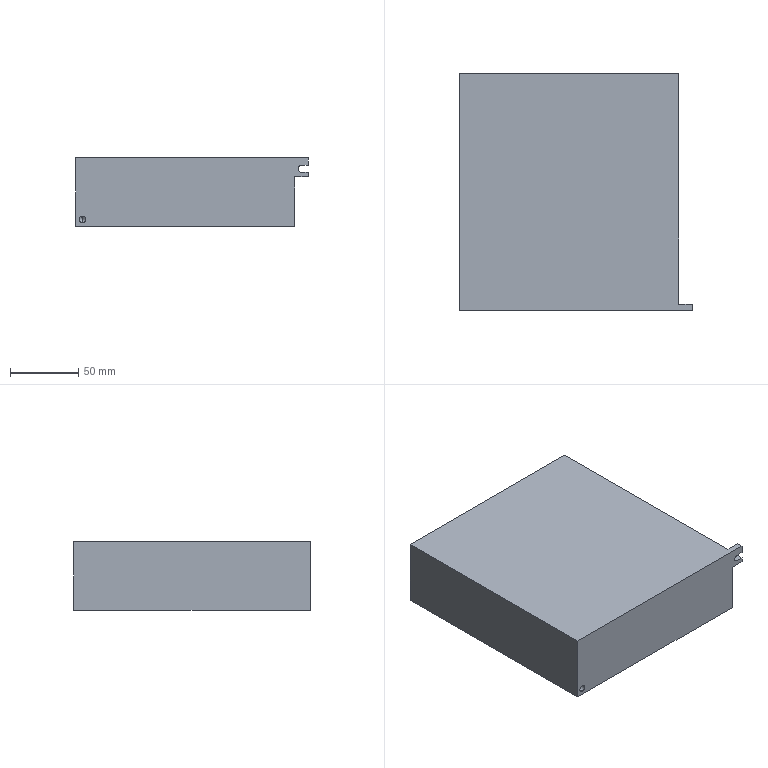Part | STEP file | Jiemeikang 750W driver | 1 solid | 17 faces | box 170 x 173 x 50 mm | volume 1384193 mm3 | plane 12 | cylinder 3 | cone 2 | commonest cylinder face diameters 4.8 x2 5 x1
STEP:
#1=CARTESIAN_POINT('',(0.,0.,0.));
#2=DIRECTION('',(0.,0.,1.));
#3=DIRECTION('',(1.,0.,0.));
#4=AXIS2_PLACEMENT_3D('',#1,#2,#3);
#5=CARTESIAN_POINT('',(-75.,15.,-22.4));
#6=VERTEX_POINT('',#5);
#7=CARTESIAN_POINT('',(-75.,0.,-22.4));
#8=VERTEX_POINT('',#7);
#9=CARTESIAN_POINT('',(-75.,0.,-22.4));
#10=DIRECTION('',(0.,-1.,0.));
#11=VECTOR('',#10,1.);
#12=LINE('',#9,#11);
#13=CARTESIAN_POINT('',(-75.,0.,-20.));
#14=DIRECTION('',(0.,-1.,0.));
#15=DIRECTION('',(0.,0.,-1.));
#16=AXIS2_PLACEMENT_3D('',#13,#14,#15);
#17=CYLINDRICAL_SURFACE('',#16,2.4);
#18=CARTESIAN_POINT('',(6.283,0.));
#19=DIRECTION('',(0.,1.));
#20=VECTOR('',#19,1.);
#21=LINE('',#18,#20);
#22=(GEOMETRIC_REPRESENTATION_CONTEXT(2)PARAMETRIC_REPRESENTATION_CONTEXT()REPRESENTATION_CONTEXT('',''));
#23=DEFINITIONAL_REPRESENTATION('',(#21),#22);
#24=PCURVE('',#17,#23);
#25=CARTESIAN_POINT('',(-75.,0.,-20.));
#26=DIRECTION('',(0.,-1.,0.));
#27=DIRECTION('',(0.,0.,-1.));
#28=AXIS2_PLACEMENT_3D('',#25,#26,#27);
#29=CYLINDRICAL_SURFACE('',#28,2.4);
#30=CARTESIAN_POINT('',(0.,0.));
#31=DIRECTION('',(0.,1.));
#32=VECTOR('',#31,1.);
#33=LINE('',#30,#32);
#34=(GEOMETRIC_REPRESENTATION_CONTEXT(2)PARAMETRIC_REPRESENTATION_CONTEXT()REPRESENTATION_CONTEXT('',''));
#35=DEFINITIONAL_REPRESENTATION('',(#33),#34);
#36=PCURVE('',#29,#35);
#37=SURFACE_CURVE('',#12,(#24,#36),.PCURVE_S1.);
#38=EDGE_CURVE('',#6,#8,#37,.T.);
#39=ORIENTED_EDGE('',*,*,#38,.T.);
#40=CARTESIAN_POINT('',(-75.,0.,-17.6));
#41=VERTEX_POINT('',#40);
#42=CARTESIAN_POINT('',(-75.,0.,-20.));
#43=DIRECTION('',(0.,-1.,0.));
#44=DIRECTION('',(0.,0.,-1.));
#45=AXIS2_PLACEMENT_3D('',#42,#43,#44);
#46=CIRCLE('',#45,2.4);
#47=CARTESIAN_POINT('',(0.,0.));
#48=DIRECTION('',(1.,0.));
#49=VECTOR('',#48,1.);
#50=LINE('',#47,#49);
#51=(GEOMETRIC_REPRESENTATION_CONTEXT(2)PARAMETRIC_REPRESENTATION_CONTEXT()REPRESENTATION_CONTEXT('',''));
#52=DEFINITIONAL_REPRESENTATION('',(#50),#51);
#53=PCURVE('',#17,#52);
#54=CARTESIAN_POINT('',(0.,0.,0.));
#55=DIRECTION('',(0.,-1.,0.));
#56=DIRECTION('',(0.,0.,-1.));
#57=AXIS2_PLACEMENT_3D('',#54,#55,#56);
#58=PLANE('',#57);
#59=CARTESIAN_POINT('',(20.,-75.));
#60=DIRECTION('',(1.,0.));
#61=AXIS2_PLACEMENT_2D('',#59,#60);
#62=CIRCLE('',#61,2.4);
#63=(GEOMETRIC_REPRESENTATION_CONTEXT(2)PARAMETRIC_REPRESENTATION_CONTEXT()REPRESENTATION_CONTEXT('',''));
#64=DEFINITIONAL_REPRESENTATION('',(#62),#63);
#65=PCURVE('',#58,#64);
#66=SURFACE_CURVE('',#46,(#53,#65),.PCURVE_S1.);
#67=EDGE_CURVE('',#41,#8,#66,.T.);
#68=ORIENTED_EDGE('',*,*,#67,.F.);
#69=CARTESIAN_POINT('',(-75.,15.,-17.6));
#70=VERTEX_POINT('',#69);
#71=CARTESIAN_POINT('',(-75.,0.,-17.6));
#72=DIRECTION('',(0.,-1.,0.));
#73=VECTOR('',#72,1.);
#74=LINE('',#71,#73);
#75=CARTESIAN_POINT('',(3.142,0.));
#76=DIRECTION('',(0.,1.));
#77=VECTOR('',#76,1.);
#78=LINE('',#75,#77);
#79=(GEOMETRIC_REPRESENTATION_CONTEXT(2)PARAMETRIC_REPRESENTATION_CONTEXT()REPRESENTATION_CONTEXT('',''));
#80=DEFINITIONAL_REPRESENTATION('',(#78),#79);
#81=PCURVE('',#17,#80);
#82=CARTESIAN_POINT('',(3.142,0.));
#83=DIRECTION('',(0.,1.));
#84=VECTOR('',#83,1.);
#85=LINE('',#82,#84);
#86=(GEOMETRIC_REPRESENTATION_CONTEXT(2)PARAMETRIC_REPRESENTATION_CONTEXT()REPRESENTATION_CONTEXT('',''));
#87=DEFINITIONAL_REPRESENTATION('',(#85),#86);
#88=PCURVE('',#29,#87);
#89=SURFACE_CURVE('',#74,(#81,#88),.PCURVE_S1.);
#90=EDGE_CURVE('',#70,#41,#89,.T.);
#91=ORIENTED_EDGE('',*,*,#90,.F.);
#92=CARTESIAN_POINT('',(-75.,15.,-20.));
#93=DIRECTION('',(0.,-1.,0.));
#94=DIRECTION('',(0.,0.,-1.));
#95=AXIS2_PLACEMENT_3D('',#92,#93,#94);
#96=CIRCLE('',#95,2.4);
#97=CARTESIAN_POINT('',(0.,-15.));
#98=DIRECTION('',(1.,0.));
#99=VECTOR('',#98,1.);
#100=LINE('',#97,#99);
#101=(GEOMETRIC_REPRESENTATION_CONTEXT(2)PARAMETRIC_REPRESENTATION_CONTEXT()REPRESENTATION_CONTEXT('',''));
#102=DEFINITIONAL_REPRESENTATION('',(#100),#101);
#103=PCURVE('',#17,#102);
#104=CARTESIAN_POINT('',(-75.,15.,-20.));
#105=DIRECTION('',(0.,-1.,0.));
#106=DIRECTION('',(0.,0.,-1.));
#107=AXIS2_PLACEMENT_3D('',#104,#105,#106);
#108=CONICAL_SURFACE('',#107,2.4,1.03);
#109=CARTESIAN_POINT('',(0.,0.));
#110=DIRECTION('',(1.,0.));
#111=VECTOR('',#110,1.);
#112=LINE('',#109,#111);
#113=(GEOMETRIC_REPRESENTATION_CONTEXT(2)PARAMETRIC_REPRESENTATION_CONTEXT()REPRESENTATION_CONTEXT('',''));
#114=DEFINITIONAL_REPRESENTATION('',(#112),#113);
#115=PCURVE('',#108,#114);
#116=SURFACE_CURVE('',#96,(#103,#115),.PCURVE_S1.);
#117=EDGE_CURVE('',#70,#6,#116,.T.);
#118=ORIENTED_EDGE('',*,*,#117,.T.);
#119=EDGE_LOOP('',(#39,#68,#91,#118));
#120=FACE_BOUND('',#119,.F.);
#121=ADVANCED_FACE('',(#120),#17,.F.);
#122=ORIENTED_EDGE('',*,*,#117,.F.);
#123=CARTESIAN_POINT('',(-75.,16.442,-20.));
#124=VERTEX_POINT('',#123);
#125=CARTESIAN_POINT('',(-75.,15.,-17.6));
#126=DIRECTION('',(0.,-0.515,0.8572));
#127=VECTOR('',#126,1.);
#128=LINE('',#125,#127);
#129=CARTESIAN_POINT('',(3.142,-1.442));
#130=CARTESIAN_POINT('',(3.142,-1.42));
#131=CARTESIAN_POINT('',(3.142,-1.377));
#132=CARTESIAN_POINT('',(3.142,-1.311));
#133=CARTESIAN_POINT('',(3.142,-1.245));
#134=CARTESIAN_POINT('',(3.142,-1.18));
#135=CARTESIAN_POINT('',(3.142,-1.114));
#136=CARTESIAN_POINT('',(3.142,-1.049));
#137=CARTESIAN_POINT('',(3.142,-0.9832));
#138=CARTESIAN_POINT('',(3.142,-0.9177));
#139=CARTESIAN_POINT('',(3.142,-0.8521));
#140=CARTESIAN_POINT('',(3.142,-0.7866));
#141=CARTESIAN_POINT('',(3.142,-0.721));
#142=CARTESIAN_POINT('',(3.142,-0.6555));
#143=CARTESIAN_POINT('',(3.142,-0.5899));
#144=CARTESIAN_POINT('',(3.142,-0.5244));
#145=CARTESIAN_POINT('',(3.142,-0.4588));
#146=CARTESIAN_POINT('',(3.142,-0.3933));
#147=CARTESIAN_POINT('',(3.142,-0.3277));
#148=CARTESIAN_POINT('',(3.142,-0.2622));
#149=CARTESIAN_POINT('',(3.142,-0.1966));
#150=CARTESIAN_POINT('',(3.142,-0.1311));
#151=CARTESIAN_POINT('',(3.142,-0.06555));
#152=CARTESIAN_POINT('',(3.142,-0.02185));
#153=CARTESIAN_POINT('',(3.142,0.));
#154=B_SPLINE_CURVE_WITH_KNOTS('',3,(#129,#130,#131,#132,#133,#134,#135,#136,#137,#138,#139,#140,#141,#142,#143,#144,#145,#146,#147,#148,#149,#150,#151,#152,#153),.UNSPECIFIED.,.F.,.F.,(4,1,1,1,1,1,1,1,1,1,1,1,1,1,1,1,1,1,1,1,1,1,4),(-2.8,-2.673,-2.545,-2.418,-2.291,-2.164,-2.036,-1.909,-1.782,-1.654,-1.527,-1.4,-1.273,-1.145,-1.018,-0.8909,-0.7636,-0.6363,-0.5091,-0.3818,-0.2545,-0.1273,0.),.UNSPECIFIED.);
#155=(GEOMETRIC_REPRESENTATION_CONTEXT(2)PARAMETRIC_REPRESENTATION_CONTEXT()REPRESENTATION_CONTEXT('',''));
#156=DEFINITIONAL_REPRESENTATION('',(#154),#155);
#157=PCURVE('',#108,#156);
#158=CARTESIAN_POINT('',(-75.,15.,-20.));
#159=DIRECTION('',(0.,-1.,0.));
#160=DIRECTION('',(0.,0.,-1.));
#161=AXIS2_PLACEMENT_3D('',#158,#159,#160);
#162=CONICAL_SURFACE('',#161,2.4,1.03);
#163=CARTESIAN_POINT('',(3.142,-1.442));
#164=CARTESIAN_POINT('',(3.142,-1.42));
#165=CARTESIAN_POINT('',(3.142,-1.377));
#166=CARTESIAN_POINT('',(3.142,-1.311));
#167=CARTESIAN_POINT('',(3.142,-1.245));
#168=CARTESIAN_POINT('',(3.142,-1.18));
#169=CARTESIAN_POINT('',(3.142,-1.114));
#170=CARTESIAN_POINT('',(3.142,-1.049));
#171=CARTESIAN_POINT('',(3.142,-0.9832));
#172=CARTESIAN_POINT('',(3.142,-0.9177));
#173=CARTESIAN_POINT('',(3.142,-0.8521));
#174=CARTESIAN_POINT('',(3.142,-0.7866));
#175=CARTESIAN_POINT('',(3.142,-0.721));
#176=CARTESIAN_POINT('',(3.142,-0.6555));
#177=CARTESIAN_POINT('',(3.142,-0.5899));
#178=CARTESIAN_POINT('',(3.142,-0.5244));
#179=CARTESIAN_POINT('',(3.142,-0.4588));
#180=CARTESIAN_POINT('',(3.142,-0.3933));
#181=CARTESIAN_POINT('',(3.142,-0.3277));
#182=CARTESIAN_POINT('',(3.142,-0.2622));
#183=CARTESIAN_POINT('',(3.142,-0.1966));
#184=CARTESIAN_POINT('',(3.142,-0.1311));
#185=CARTESIAN_POINT('',(3.142,-0.06555));
#186=CARTESIAN_POINT('',(3.142,-0.02185));
#187=CARTESIAN_POINT('',(3.142,0.));
#188=B_SPLINE_CURVE_WITH_KNOTS('',3,(#163,#164,#165,#166,#167,#168,#169,#170,#171,#172,#173,#174,#175,#176,#177,#178,#179,#180,#181,#182,#183,#184,#185,#186,#187),.UNSPECIFIED.,.F.,.F.,(4,1,1,1,1,1,1,1,1,1,1,1,1,1,1,1,1,1,1,1,1,1,4),(-2.8,-2.673,-2.545,-2.418,-2.291,-2.164,-2.036,-1.909,-1.782,-1.654,-1.527,-1.4,-1.273,-1.145,-1.018,-0.8909,-0.7636,-0.6363,-0.5091,-0.3818,-0.2545,-0.1273,0.),.UNSPECIFIED.);
#189=(GEOMETRIC_REPRESENTATION_CONTEXT(2)PARAMETRIC_REPRESENTATION_CONTEXT()REPRESENTATION_CONTEXT('',''));
#190=DEFINITIONAL_REPRESENTATION('',(#188),#189);
#191=PCURVE('',#162,#190);
#192=SURFACE_CURVE('',#128,(#157,#191),.PCURVE_S1.);
#193=EDGE_CURVE('',#124,#70,#192,.T.);
#194=ORIENTED_EDGE('',*,*,#193,.F.);
#195=CARTESIAN_POINT('',(-75.,15.,-22.4));
#196=DIRECTION('',(0.,-0.515,-0.8572));
#197=VECTOR('',#196,1.);
#198=LINE('',#195,#197);
#199=CARTESIAN_POINT('',(6.283,0.));
#200=DIRECTION('',(0.,1.));
#201=VECTOR('',#200,1.);
#202=LINE('',#199,#201);
#203=(GEOMETRIC_REPRESENTATION_CONTEXT(2)PARAMETRIC_REPRESENTATION_CONTEXT()REPRESENTATION_CONTEXT('',''));
#204=DEFINITIONAL_REPRESENTATION('',(#202),#203);
#205=PCURVE('',#108,#204);
#206=CARTESIAN_POINT('',(0.,0.));
#207=DIRECTION('',(0.,1.));
#208=VECTOR('',#207,1.);
#209=LINE('',#206,#208);
#210=(GEOMETRIC_REPRESENTATION_CONTEXT(2)PARAMETRIC_REPRESENTATION_CONTEXT()REPRESENTATION_CONTEXT('',''));
#211=DEFINITIONAL_REPRESENTATION('',(#209),#210);
#212=PCURVE('',#162,#211);
#213=SURFACE_CURVE('',#198,(#205,#212),.PCURVE_S1.);
#214=EDGE_CURVE('',#124,#6,#213,.T.);
#215=ORIENTED_EDGE('',*,*,#214,.T.);
#216=EDGE_LOOP('',(#122,#194,#215));
#217=FACE_BOUND('',#216,.F.);
#218=ADVANCED_FACE('',(#217),#108,.F.);
#219=CARTESIAN_POINT('',(90.,0.,14.5));
#220=VERTEX_POINT('',#219);
#221=CARTESIAN_POINT('',(90.,4.5,14.5));
#222=VERTEX_POINT('',#221);
#223=CARTESIAN_POINT('',(90.,0.,14.5));
#224=DIRECTION('',(0.,1.,0.));
#225=VECTOR('',#224,1.);
#226=LINE('',#223,#225);
#227=CARTESIAN_POINT('',(90.,4.5,25.));
#228=DIRECTION('',(1.,0.,0.));
#229=DIRECTION('',(0.,0.,-1.));
#230=AXIS2_PLACEMENT_3D('',#227,#228,#229);
#231=PLANE('',#230);
#232=CARTESIAN_POINT('',(10.5,-4.5));
#233=DIRECTION('',(0.,1.));
#234=VECTOR('',#233,1.);
#235=LINE('',#232,#234);
#236=(GEOMETRIC_REPRESENTATION_CONTEXT(2)PARAMETRIC_REPRESENTATION_CONTEXT()REPRESENTATION_CONTEXT('',''));
#237=DEFINITIONAL_REPRESENTATION('',(#235),#236);
#238=PCURVE('',#231,#237);
#239=CARTESIAN_POINT('',(85.,0.,14.5));
#240=DIRECTION('',(0.,0.,-1.));
#241=DIRECTION('',(-1.,0.,0.));
#242=AXIS2_PLACEMENT_3D('',#239,#240,#241);
#243=PLANE('',#242);
#244=CARTESIAN_POINT('',(-5.,0.));
#245=DIRECTION('',(0.,1.));
#246=VECTOR('',#245,1.);
#247=LINE('',#244,#246);
#248=(GEOMETRIC_REPRESENTATION_CONTEXT(2)PARAMETRIC_REPRESENTATION_CONTEXT()REPRESENTATION_CONTEXT('',''));
#249=DEFINITIONAL_REPRESENTATION('',(#247),#248);
#250=PCURVE('',#243,#249);
#251=SURFACE_CURVE('',#226,(#238,#250),.PCURVE_S1.);
#252=EDGE_CURVE('',#220,#222,#251,.T.);
#253=ORIENTED_EDGE('',*,*,#252,.F.);
#254=CARTESIAN_POINT('',(90.,0.,11.));
#255=VERTEX_POINT('',#254);
#256=CARTESIAN_POINT('',(90.,0.,25.));
#257=DIRECTION('',(0.,0.,1.));
#258=VECTOR('',#257,1.);
#259=LINE('',#256,#258);
#260=CARTESIAN_POINT('',(0.,-4.5));
#261=DIRECTION('',(-1.,0.));
#262=VECTOR('',#261,1.);
#263=LINE('',#260,#262);
#264=(GEOMETRIC_REPRESENTATION_CONTEXT(2)PARAMETRIC_REPRESENTATION_CONTEXT()REPRESENTATION_CONTEXT('',''));
#265=DEFINITIONAL_REPRESENTATION('',(#263),#264);
#266=PCURVE('',#231,#265);
#267=CARTESIAN_POINT('',(-25.,90.));
#268=DIRECTION('',(-1.,0.));
#269=VECTOR('',#268,1.);
#270=LINE('',#267,#269);
#271=(GEOMETRIC_REPRESENTATION_CONTEXT(2)PARAMETRIC_REPRESENTATION_CONTEXT()REPRESENTATION_CONTEXT('',''));
#272=DEFINITIONAL_REPRESENTATION('',(#270),#271);
#273=PCURVE('',#58,#272);
#274=SURFACE_CURVE('',#259,(#266,#273),.PCURVE_S1.);
#275=EDGE_CURVE('',#255,#220,#274,.T.);
#276=ORIENTED_EDGE('',*,*,#275,.F.);
#277=CARTESIAN_POINT('',(90.,4.5,11.));
#278=VERTEX_POINT('',#277);
#279=CARTESIAN_POINT('',(90.,4.5,11.));
#280=DIRECTION('',(0.,-1.,0.));
#281=VECTOR('',#280,1.);
#282=LINE('',#279,#281);
#283=CARTESIAN_POINT('',(14.,0.));
#284=DIRECTION('',(0.,-1.));
#285=VECTOR('',#284,1.);
#286=LINE('',#283,#285);
#287=(GEOMETRIC_REPRESENTATION_CONTEXT(2)PARAMETRIC_REPRESENTATION_CONTEXT()REPRESENTATION_CONTEXT('',''));
#288=DEFINITIONAL_REPRESENTATION('',(#286),#287);
#289=PCURVE('',#231,#288);
#290=CARTESIAN_POINT('',(80.,4.5,11.));
#291=DIRECTION('',(0.,0.,-1.));
#292=DIRECTION('',(-1.,0.,0.));
#293=AXIS2_PLACEMENT_3D('',#290,#291,#292);
#294=PLANE('',#293);
#295=CARTESIAN_POINT('',(-10.,0.));
#296=DIRECTION('',(0.,-1.));
#297=VECTOR('',#296,1.);
#298=LINE('',#295,#297);
#299=(GEOMETRIC_REPRESENTATION_CONTEXT(2)PARAMETRIC_REPRESENTATION_CONTEXT()REPRESENTATION_CONTEXT('',''));
#300=DEFINITIONAL_REPRESENTATION('',(#298),#299);
#301=PCURVE('',#294,#300);
#302=SURFACE_CURVE('',#282,(#289,#301),.PCURVE_S1.);
#303=EDGE_CURVE('',#278,#255,#302,.T.);
#304=ORIENTED_EDGE('',*,*,#303,.F.);
#305=CARTESIAN_POINT('',(90.,4.5,25.));
#306=DIRECTION('',(0.,0.,1.));
#307=VECTOR('',#306,1.);
#308=LINE('',#305,#307);
#309=CARTESIAN_POINT('',(0.,0.));
#310=DIRECTION('',(-1.,0.));
#311=VECTOR('',#310,1.);
#312=LINE('',#309,#311);
#313=(GEOMETRIC_REPRESENTATION_CONTEXT(2)PARAMETRIC_REPRESENTATION_CONTEXT()REPRESENTATION_CONTEXT('',''));
#314=DEFINITIONAL_REPRESENTATION('',(#312),#313);
#315=PCURVE('',#231,#314);
#316=CARTESIAN_POINT('',(0.,4.5,0.));
#317=DIRECTION('',(0.,-1.,0.));
#318=DIRECTION('',(0.,0.,-1.));
#319=AXIS2_PLACEMENT_3D('',#316,#317,#318);
#320=PLANE('',#319);
#321=CARTESIAN_POINT('',(-25.,90.));
#322=DIRECTION('',(-1.,0.));
#323=VECTOR('',#322,1.);
#324=LINE('',#321,#323);
#325=(GEOMETRIC_REPRESENTATION_CONTEXT(2)PARAMETRIC_REPRESENTATION_CONTEXT()REPRESENTATION_CONTEXT('',''));
#326=DEFINITIONAL_REPRESENTATION('',(#324),#325);
#327=PCURVE('',#320,#326);
#328=SURFACE_CURVE('',#308,(#315,#327),.PCURVE_S1.);
#329=EDGE_CURVE('',#278,#222,#328,.T.);
#330=ORIENTED_EDGE('',*,*,#329,.T.);
#331=EDGE_LOOP('',(#253,#276,#304,#330));
#332=FACE_BOUND('',#331,.T.);
#333=ADVANCED_FACE('',(#332),#231,.T.);
#334=CARTESIAN_POINT('',(80.,173.,25.));
#335=VERTEX_POINT('',#334);
#336=CARTESIAN_POINT('',(80.,4.5,25.));
#337=VERTEX_POINT('',#336);
#338=CARTESIAN_POINT('',(80.,173.,25.));
#339=DIRECTION('',(0.,-1.,0.));
#340=VECTOR('',#339,1.);
#341=LINE('',#338,#340);
#342=CARTESIAN_POINT('',(80.,173.,25.));
#343=DIRECTION('',(-1.,0.,0.));
#344=DIRECTION('',(0.,0.,1.));
#345=AXIS2_PLACEMENT_3D('',#342,#343,#344);
#346=PLANE('',#345);
#347=CARTESIAN_POINT('',(0.,0.));
#348=DIRECTION('',(0.,-1.));
#349=VECTOR('',#348,1.);
#350=LINE('',#347,#349);
#351=(GEOMETRIC_REPRESENTATION_CONTEXT(2)PARAMETRIC_REPRESENTATION_CONTEXT()REPRESENTATION_CONTEXT('',''));
#352=DEFINITIONAL_REPRESENTATION('',(#350),#351);
#353=PCURVE('',#346,#352);
#354=CARTESIAN_POINT('',(-80.,173.,25.));
#355=DIRECTION('',(0.,0.,-1.));
#356=DIRECTION('',(-1.,0.,0.));
#357=AXIS2_PLACEMENT_3D('',#354,#355,#356);
#358=PLANE('',#357);
#359=CARTESIAN_POINT('',(-160.,0.));
#360=DIRECTION('',(0.,-1.));
#361=VECTOR('',#360,1.);
#362=LINE('',#359,#361);
#363=(GEOMETRIC_REPRESENTATION_CONTEXT(2)PARAMETRIC_REPRESENTATION_CONTEXT()REPRESENTATION_CONTEXT('',''));
#364=DEFINITIONAL_REPRESENTATION('',(#362),#363);
#365=PCURVE('',#358,#364);
#366=SURFACE_CURVE('',#341,(#353,#365),.PCURVE_S1.);
#367=EDGE_CURVE('',#335,#337,#366,.T.);
#368=ORIENTED_EDGE('',*,*,#367,.T.);
#369=CARTESIAN_POINT('',(80.,4.5,11.));
#370=VERTEX_POINT('',#369);
#371=CARTESIAN_POINT('',(80.,4.5,25.));
#372=DIRECTION('',(0.,0.,-1.));
#373=VECTOR('',#372,1.);
#374=LINE('',#371,#373);
#375=CARTESIAN_POINT('',(0.,-168.5));
#376=DIRECTION('',(-1.,0.));
#377=VECTOR('',#376,1.);
#378=LINE('',#375,#377);
#379=(GEOMETRIC_REPRESENTATION_CONTEXT(2)PARAMETRIC_REPRESENTATION_CONTEXT()REPRESENTATION_CONTEXT('',''));
#380=DEFINITIONAL_REPRESENTATION('',(#378),#379);
#381=PCURVE('',#346,#380);
#382=CARTESIAN_POINT('',(-25.,80.));
#383=DIRECTION('',(1.,0.));
#384=VECTOR('',#383,1.);
#385=LINE('',#382,#384);
#386=(GEOMETRIC_REPRESENTATION_CONTEXT(2)PARAMETRIC_REPRESENTATION_CONTEXT()REPRESENTATION_CONTEXT('',''));
#387=DEFINITIONAL_REPRESENTATION('',(#385),#386);
#388=PCURVE('',#320,#387);
#389=SURFACE_CURVE('',#374,(#381,#388),.PCURVE_S1.);
#390=EDGE_CURVE('',#337,#370,#389,.T.);
#391=ORIENTED_EDGE('',*,*,#390,.T.);
#392=CARTESIAN_POINT('',(80.,0.,11.));
#393=VERTEX_POINT('',#392);
#394=CARTESIAN_POINT('',(80.,4.5,11.));
#395=DIRECTION('',(0.,-1.,0.));
#396=VECTOR('',#395,1.);
#397=LINE('',#394,#396);
#398=CARTESIAN_POINT('',(-14.,-168.5));
#399=DIRECTION('',(0.,-1.));
#400=VECTOR('',#399,1.);
#401=LINE('',#398,#400);
#402=(GEOMETRIC_REPRESENTATION_CONTEXT(2)PARAMETRIC_REPRESENTATION_CONTEXT()REPRESENTATION_CONTEXT('',''));
#403=DEFINITIONAL_REPRESENTATION('',(#401),#402);
#404=PCURVE('',#346,#403);
#405=CARTESIAN_POINT('',(0.,0.));
#406=DIRECTION('',(0.,-1.));
#407=VECTOR('',#406,1.);
#408=LINE('',#405,#407);
#409=(GEOMETRIC_REPRESENTATION_CONTEXT(2)PARAMETRIC_REPRESENTATION_CONTEXT()REPRESENTATION_CONTEXT('',''));
#410=DEFINITIONAL_REPRESENTATION('',(#408),#409);
#411=PCURVE('',#294,#410);
#412=SURFACE_CURVE('',#397,(#404,#411),.PCURVE_S1.);
#413=EDGE_CURVE('',#370,#393,#412,.T.);
#414=ORIENTED_EDGE('',*,*,#413,.T.);
#415=CARTESIAN_POINT('',(80.,0.,-25.));
#416=VERTEX_POINT('',#415);
#417=CARTESIAN_POINT('',(80.,0.,25.));
#418=DIRECTION('',(0.,0.,-1.));
#419=VECTOR('',#418,1.);
#420=LINE('',#417,#419);
#421=CARTESIAN_POINT('',(0.,-173.));
#422=DIRECTION('',(-1.,0.));
#423=VECTOR('',#422,1.);
#424=LINE('',#421,#423);
#425=(GEOMETRIC_REPRESENTATION_CONTEXT(2)PARAMETRIC_REPRESENTATION_CONTEXT()REPRESENTATION_CONTEXT('',''));
#426=DEFINITIONAL_REPRESENTATION('',(#424),#425);
#427=PCURVE('',#346,#426);
#428=CARTESIAN_POINT('',(-25.,80.));
#429=DIRECTION('',(1.,0.));
#430=VECTOR('',#429,1.);
#431=LINE('',#428,#430);
#432=(GEOMETRIC_REPRESENTATION_CONTEXT(2)PARAMETRIC_REPRESENTATION_CONTEXT()REPRESENTATION_CONTEXT('',''));
#433=DEFINITIONAL_REPRESENTATION('',(#431),#432);
#434=PCURVE('',#58,#433);
#435=SURFACE_CURVE('',#420,(#427,#434),.PCURVE_S1.);
#436=EDGE_CURVE('',#393,#416,#435,.T.);
#437=ORIENTED_EDGE('',*,*,#436,.T.);
#438=CARTESIAN_POINT('',(80.,173.,-25.));
#439=VERTEX_POINT('',#438);
#440=CARTESIAN_POINT('',(80.,173.,-25.));
#441=DIRECTION('',(0.,-1.,0.));
#442=VECTOR('',#441,1.);
#443=LINE('',#440,#442);
#444=CARTESIAN_POINT('',(-50.,0.));
#445=DIRECTION('',(0.,-1.));
#446=VECTOR('',#445,1.);
#447=LINE('',#444,#446);
#448=(GEOMETRIC_REPRESENTATION_CONTEXT(2)PARAMETRIC_REPRESENTATION_CONTEXT()REPRESENTATION_CONTEXT('',''));
#449=DEFINITIONAL_REPRESENTATION('',(#447),#448);
#450=PCURVE('',#346,#449);
#451=CARTESIAN_POINT('',(-80.,173.,-25.));
#452=DIRECTION('',(0.,0.,1.));
#453=DIRECTION('',(1.,0.,0.));
#454=AXIS2_PLACEMENT_3D('',#451,#452,#453);
#455=PLANE('',#454);
#456=CARTESIAN_POINT('',(160.,0.));
#457=DIRECTION('',(0.,-1.));
#458=VECTOR('',#457,1.);
#459=LINE('',#456,#458);
#460=(GEOMETRIC_REPRESENTATION_CONTEXT(2)PARAMETRIC_REPRESENTATION_CONTEXT()REPRESENTATION_CONTEXT('',''));
#461=DEFINITIONAL_REPRESENTATION('',(#459),#460);
#462=PCURVE('',#455,#461);
#463=SURFACE_CURVE('',#443,(#450,#462),.PCURVE_S1.);
#464=EDGE_CURVE('',#439,#416,#463,.T.);
#465=ORIENTED_EDGE('',*,*,#464,.F.);
#466=CARTESIAN_POINT('',(80.,173.,25.));
#467=DIRECTION('',(0.,0.,-1.));
#468=VECTOR('',#467,1.);
#469=LINE('',#466,#468);
#470=CARTESIAN_POINT('',(0.,0.));
#471=DIRECTION('',(-1.,0.));
#472=VECTOR('',#471,1.);
#473=LINE('',#470,#472);
#474=(GEOMETRIC_REPRESENTATION_CONTEXT(2)PARAMETRIC_REPRESENTATION_CONTEXT()REPRESENTATION_CONTEXT('',''));
#475=DEFINITIONAL_REPRESENTATION('',(#473),#474);
#476=PCURVE('',#346,#475);
#477=CARTESIAN_POINT('',(0.,173.,0.));
#478=DIRECTION('',(0.,-1.,0.));
#479=DIRECTION('',(0.,0.,-1.));
#480=AXIS2_PLACEMENT_3D('',#477,#478,#479);
#481=PLANE('',#480);
#482=CARTESIAN_POINT('',(-25.,80.));
#483=DIRECTION('',(1.,0.));
#484=VECTOR('',#483,1.);
#485=LINE('',#482,#484);
#486=(GEOMETRIC_REPRESENTATION_CONTEXT(2)PARAMETRIC_REPRESENTATION_CONTEXT()REPRESENTATION_CONTEXT('',''));
#487=DEFINITIONAL_REPRESENTATION('',(#485),#486);
#488=PCURVE('',#481,#487);
#489=SURFACE_CURVE('',#469,(#476,#488),.PCURVE_S1.);
#490=EDGE_CURVE('',#335,#439,#489,.T.);
#491=ORIENTED_EDGE('',*,*,#490,.F.);
#492=EDGE_LOOP('',(#368,#391,#414,#437,#465,#491));
#493=FACE_BOUND('',#492,.T.);
#494=ADVANCED_FACE('',(#493),#346,.F.);
#495=CARTESIAN_POINT('',(-80.,0.,-25.));
#496=VERTEX_POINT('',#495);
#497=CARTESIAN_POINT('',(-80.,0.,-25.));
#498=DIRECTION('',(-1.,0.,0.));
#499=VECTOR('',#498,1.);
#500=LINE('',#497,#499);
#501=CARTESIAN_POINT('',(0.,-173.));
#502=DIRECTION('',(-1.,0.));
#503=VECTOR('',#502,1.);
#504=LINE('',#501,#503);
#505=(GEOMETRIC_REPRESENTATION_CONTEXT(2)PARAMETRIC_REPRESENTATION_CONTEXT()REPRESENTATION_CONTEXT('',''));
#506=DEFINITIONAL_REPRESENTATION('',(#504),#505);
#507=PCURVE('',#455,#506);
#508=CARTESIAN_POINT('',(25.,-80.));
#509=DIRECTION('',(0.,-1.));
#510=VECTOR('',#509,1.);
#511=LINE('',#508,#510);
#512=(GEOMETRIC_REPRESENTATION_CONTEXT(2)PARAMETRIC_REPRESENTATION_CONTEXT()REPRESENTATION_CONTEXT('',''));
#513=DEFINITIONAL_REPRESENTATION('',(#511),#512);
#514=PCURVE('',#58,#513);
#515=SURFACE_CURVE('',#500,(#507,#514),.PCURVE_S1.);
#516=EDGE_CURVE('',#416,#496,#515,.T.);
#517=ORIENTED_EDGE('',*,*,#516,.T.);
#518=CARTESIAN_POINT('',(-80.,173.,-25.));
#519=VERTEX_POINT('',#518);
#520=CARTESIAN_POINT('',(-80.,173.,-25.));
#521=DIRECTION('',(0.,-1.,0.));
#522=VECTOR('',#521,1.);
#523=LINE('',#520,#522);
#524=CARTESIAN_POINT('',(0.,0.));
#525=DIRECTION('',(0.,-1.));
#526=VECTOR('',#525,1.);
#527=LINE('',#524,#526);
#528=(GEOMETRIC_REPRESENTATION_CONTEXT(2)PARAMETRIC_REPRESENTATION_CONTEXT()REPRESENTATION_CONTEXT('',''));
#529=DEFINITIONAL_REPRESENTATION('',(#527),#528);
#530=PCURVE('',#455,#529);
#531=CARTESIAN_POINT('',(-80.,173.,25.));
#532=DIRECTION('',(1.,0.,0.));
#533=DIRECTION('',(0.,0.,-1.));
#534=AXIS2_PLACEMENT_3D('',#531,#532,#533);
#535=PLANE('',#534);
#536=CARTESIAN_POINT('',(50.,0.));
#537=DIRECTION('',(0.,-1.));
#538=VECTOR('',#537,1.);
#539=LINE('',#536,#538);
#540=(GEOMETRIC_REPRESENTATION_CONTEXT(2)PARAMETRIC_REPRESENTATION_CONTEXT()REPRESENTATION_CONTEXT('',''));
#541=DEFINITIONAL_REPRESENTATION('',(#539),#540);
#542=PCURVE('',#535,#541);
#543=SURFACE_CURVE('',#523,(#530,#542),.PCURVE_S1.);
#544=EDGE_CURVE('',#519,#496,#543,.T.);
#545=ORIENTED_EDGE('',*,*,#544,.F.);
#546=CARTESIAN_POINT('',(-80.,173.,-25.));
#547=DIRECTION('',(-1.,0.,0.));
#548=VECTOR('',#547,1.);
#549=LINE('',#546,#548);
#550=CARTESIAN_POINT('',(0.,0.));
#551=DIRECTION('',(-1.,0.));
#552=VECTOR('',#551,1.);
#553=LINE('',#550,#552);
#554=(GEOMETRIC_REPRESENTATION_CONTEXT(2)PARAMETRIC_REPRESENTATION_CONTEXT()REPRESENTATION_CONTEXT('',''));
#555=DEFINITIONAL_REPRESENTATION('',(#553),#554);
#556=PCURVE('',#455,#555);
#557=CARTESIAN_POINT('',(25.,-80.));
#558=DIRECTION('',(0.,-1.));
#559=VECTOR('',#558,1.);
#560=LINE('',#557,#559);
#561=(GEOMETRIC_REPRESENTATION_CONTEXT(2)PARAMETRIC_REPRESENTATION_CONTEXT()REPRESENTATION_CONTEXT('',''));
#562=DEFINITIONAL_REPRESENTATION('',(#560),#561);
#563=PCURVE('',#481,#562);
#564=SURFACE_CURVE('',#549,(#556,#563),.PCURVE_S1.);
#565=EDGE_CURVE('',#439,#519,#564,.T.);
#566=ORIENTED_EDGE('',*,*,#565,.F.);
#567=ORIENTED_EDGE('',*,*,#464,.T.);
#568=EDGE_LOOP('',(#517,#545,#566,#567));
#569=FACE_BOUND('',#568,.T.);
#570=ADVANCED_FACE('',(#569),#455,.F.);
#571=CARTESIAN_POINT('',(-80.,0.,25.));
#572=VERTEX_POINT('',#571);
#573=CARTESIAN_POINT('',(-80.,0.,25.));
#574=DIRECTION('',(0.,0.,1.));
#575=VECTOR('',#574,1.);
#576=LINE('',#573,#575);
#577=CARTESIAN_POINT('',(0.,-173.));
#578=DIRECTION('',(-1.,0.));
#579=VECTOR('',#578,1.);
#580=LINE('',#577,#579);
#581=(GEOMETRIC_REPRESENTATION_CONTEXT(2)PARAMETRIC_REPRESENTATION_CONTEXT()REPRESENTATION_CONTEXT('',''));
#582=DEFINITIONAL_REPRESENTATION('',(#580),#581);
#583=PCURVE('',#535,#582);
#584=CARTESIAN_POINT('',(-25.,-80.));
#585=DIRECTION('',(-1.,0.));
#586=VECTOR('',#585,1.);
#587=LINE('',#584,#586);
#588=(GEOMETRIC_REPRESENTATION_CONTEXT(2)PARAMETRIC_REPRESENTATION_CONTEXT()REPRESENTATION_CONTEXT('',''));
#589=DEFINITIONAL_REPRESENTATION('',(#587),#588);
#590=PCURVE('',#58,#589);
#591=SURFACE_CURVE('',#576,(#583,#590),.PCURVE_S1.);
#592=EDGE_CURVE('',#496,#572,#591,.T.);
#593=ORIENTED_EDGE('',*,*,#592,.T.);
#594=CARTESIAN_POINT('',(-80.,173.,25.));
#595=VERTEX_POINT('',#594);
#596=CARTESIAN_POINT('',(-80.,173.,25.));
#597=DIRECTION('',(0.,-1.,0.));
#598=VECTOR('',#597,1.);
#599=LINE('',#596,#598);
#600=CARTESIAN_POINT('',(0.,0.));
#601=DIRECTION('',(0.,-1.));
#602=VECTOR('',#601,1.);
#603=LINE('',#600,#602);
#604=(GEOMETRIC_REPRESENTATION_CONTEXT(2)PARAMETRIC_REPRESENTATION_CONTEXT()REPRESENTATION_CONTEXT('',''));
#605=DEFINITIONAL_REPRESENTATION('',(#603),#604);
#606=PCURVE('',#535,#605);
#607=CARTESIAN_POINT('',(0.,0.));
#608=DIRECTION('',(0.,-1.));
#609=VECTOR('',#608,1.);
#610=LINE('',#607,#609);
#611=(GEOMETRIC_REPRESENTATION_CONTEXT(2)PARAMETRIC_REPRESENTATION_CONTEXT()REPRESENTATION_CONTEXT('',''));
#612=DEFINITIONAL_REPRESENTATION('',(#610),#611);
#613=PCURVE('',#358,#612);
#614=SURFACE_CURVE('',#599,(#606,#613),.PCURVE_S1.);
#615=EDGE_CURVE('',#595,#572,#614,.T.);
#616=ORIENTED_EDGE('',*,*,#615,.F.);
#617=CARTESIAN_POINT('',(-80.,173.,25.));
#618=DIRECTION('',(0.,0.,1.));
#619=VECTOR('',#618,1.);
#620=LINE('',#617,#619);
#621=CARTESIAN_POINT('',(0.,0.));
#622=DIRECTION('',(-1.,0.));
#623=VECTOR('',#622,1.);
#624=LINE('',#621,#623);
#625=(GEOMETRIC_REPRESENTATION_CONTEXT(2)PARAMETRIC_REPRESENTATION_CONTEXT()REPRESENTATION_CONTEXT('',''));
#626=DEFINITIONAL_REPRESENTATION('',(#624),#625);
#627=PCURVE('',#535,#626);
#628=CARTESIAN_POINT('',(-25.,-80.));
#629=DIRECTION('',(-1.,0.));
#630=VECTOR('',#629,1.);
#631=LINE('',#628,#630);
#632=(GEOMETRIC_REPRESENTATION_CONTEXT(2)PARAMETRIC_REPRESENTATION_CONTEXT()REPRESENTATION_CONTEXT('',''));
#633=DEFINITIONAL_REPRESENTATION('',(#631),#632);
#634=PCURVE('',#481,#633);
#635=SURFACE_CURVE('',#620,(#627,#634),.PCURVE_S1.);
#636=EDGE_CURVE('',#519,#595,#635,.T.);
#637=ORIENTED_EDGE('',*,*,#636,.F.);
#638=ORIENTED_EDGE('',*,*,#544,.T.);
#639=EDGE_LOOP('',(#593,#616,#637,#638));
#640=FACE_BOUND('',#639,.T.);
#641=ADVANCED_FACE('',(#640),#535,.F.);
#642=CARTESIAN_POINT('',(90.,0.,25.));
#643=VERTEX_POINT('',#642);
#644=CARTESIAN_POINT('',(-80.,0.,25.));
#645=DIRECTION('',(1.,0.,0.));
#646=VECTOR('',#645,1.);
#647=LINE('',#644,#646);
#648=CARTESIAN_POINT('',(0.,-173.));
#649=DIRECTION('',(-1.,0.));
#650=VECTOR('',#649,1.);
#651=LINE('',#648,#650);
#652=(GEOMETRIC_REPRESENTATION_CONTEXT(2)PARAMETRIC_REPRESENTATION_CONTEXT()REPRESENTATION_CONTEXT('',''));
#653=DEFINITIONAL_REPRESENTATION('',(#651),#652);
#654=PCURVE('',#358,#653);
#655=CARTESIAN_POINT('',(-25.,-80.));
#656=DIRECTION('',(0.,1.));
#657=VECTOR('',#656,1.);
#658=LINE('',#655,#657);
#659=(GEOMETRIC_REPRESENTATION_CONTEXT(2)PARAMETRIC_REPRESENTATION_CONTEXT()REPRESENTATION_CONTEXT('',''));
#660=DEFINITIONAL_REPRESENTATION('',(#658),#659);
#661=PCURVE('',#58,#660);
#662=SURFACE_CURVE('',#647,(#654,#661),.PCURVE_S1.);
#663=EDGE_CURVE('',#572,#643,#662,.T.);
#664=ORIENTED_EDGE('',*,*,#663,.T.);
#665=CARTESIAN_POINT('',(90.,4.5,25.));
#666=VERTEX_POINT('',#665);
#667=CARTESIAN_POINT('',(90.,4.5,25.));
#668=DIRECTION('',(0.,-1.,0.));
#669=VECTOR('',#668,1.);
#670=LINE('',#667,#669);
#671=CARTESIAN_POINT('',(-170.,-168.5));
#672=DIRECTION('',(0.,-1.));
#673=VECTOR('',#672,1.);
#674=LINE('',#671,#673);
#675=(GEOMETRIC_REPRESENTATION_CONTEXT(2)PARAMETRIC_REPRESENTATION_CONTEXT()REPRESENTATION_CONTEXT('',''));
#676=DEFINITIONAL_REPRESENTATION('',(#674),#675);
#677=PCURVE('',#358,#676);
#678=CARTESIAN_POINT('',(90.,4.5,25.));
#679=DIRECTION('',(1.,0.,0.));
#680=DIRECTION('',(0.,0.,-1.));
#681=AXIS2_PLACEMENT_3D('',#678,#679,#680);
#682=PLANE('',#681);
#683=CARTESIAN_POINT('',(0.,0.));
#684=DIRECTION('',(0.,-1.));
#685=VECTOR('',#684,1.);
#686=LINE('',#683,#685);
#687=(GEOMETRIC_REPRESENTATION_CONTEXT(2)PARAMETRIC_REPRESENTATION_CONTEXT()REPRESENTATION_CONTEXT('',''));
#688=DEFINITIONAL_REPRESENTATION('',(#686),#687);
#689=PCURVE('',#682,#688);
#690=SURFACE_CURVE('',#670,(#677,#689),.PCURVE_S1.);
#691=EDGE_CURVE('',#666,#643,#690,.T.);
#692=ORIENTED_EDGE('',*,*,#691,.F.);
#693=CARTESIAN_POINT('',(80.,4.5,25.));
#694=DIRECTION('',(-1.,0.,0.));
#695=VECTOR('',#694,1.);
#696=LINE('',#693,#695);
#697=CARTESIAN_POINT('',(-160.,-168.5));
#698=DIRECTION('',(1.,0.));
#699=VECTOR('',#698,1.);
#700=LINE('',#697,#699);
#701=(GEOMETRIC_REPRESENTATION_CONTEXT(2)PARAMETRIC_REPRESENTATION_CONTEXT()REPRESENTATION_CONTEXT('',''));
#702=DEFINITIONAL_REPRESENTATION('',(#700),#701);
#703=PCURVE('',#358,#702);
#704=CARTESIAN_POINT('',(-25.,80.));
#705=DIRECTION('',(0.,-1.));
#706=VECTOR('',#705,1.);
#707=LINE('',#704,#706);
#708=(GEOMETRIC_REPRESENTATION_CONTEXT(2)PARAMETRIC_REPRESENTATION_CONTEXT()REPRESENTATION_CONTEXT('',''));
#709=DEFINITIONAL_REPRESENTATION('',(#707),#708);
#710=PCURVE('',#320,#709);
#711=SURFACE_CURVE('',#696,(#703,#710),.PCURVE_S1.);
#712=EDGE_CURVE('',#666,#337,#711,.T.);
#713=ORIENTED_EDGE('',*,*,#712,.T.);
#714=ORIENTED_EDGE('',*,*,#367,.F.);
#715=CARTESIAN_POINT('',(-80.,173.,25.));
#716=DIRECTION('',(1.,0.,0.));
#717=VECTOR('',#716,1.);
#718=LINE('',#715,#717);
#719=CARTESIAN_POINT('',(0.,0.));
#720=DIRECTION('',(-1.,0.));
#721=VECTOR('',#720,1.);
#722=LINE('',#719,#721);
#723=(GEOMETRIC_REPRESENTATION_CONTEXT(2)PARAMETRIC_REPRESENTATION_CONTEXT()REPRESENTATION_CONTEXT('',''));
#724=DEFINITIONAL_REPRESENTATION('',(#722),#723);
#725=PCURVE('',#358,#724);
#726=CARTESIAN_POINT('',(-25.,-80.));
#727=DIRECTION('',(0.,1.));
#728=VECTOR('',#727,1.);
#729=LINE('',#726,#728);
#730=(GEOMETRIC_REPRESENTATION_CONTEXT(2)PARAMETRIC_REPRESENTATION_CONTEXT()REPRESENTATION_CONTEXT('',''));
#731=DEFINITIONAL_REPRESENTATION('',(#729),#730);
#732=PCURVE('',#481,#731);
#733=SURFACE_CURVE('',#718,(#725,#732),.PCURVE_S1.);
#734=EDGE_CURVE('',#595,#335,#733,.T.);
#735=ORIENTED_EDGE('',*,*,#734,.F.);
#736=ORIENTED_EDGE('',*,*,#615,.T.);
#737=EDGE_LOOP('',(#664,#692,#713,#714,#735,#736));
#738=FACE_BOUND('',#737,.T.);
#739=ADVANCED_FACE('',(#738),#358,.F.);
#740=ORIENTED_EDGE('',*,*,#490,.T.);
#741=ORIENTED_EDGE('',*,*,#565,.T.);
#742=ORIENTED_EDGE('',*,*,#636,.T.);
#743=ORIENTED_EDGE('',*,*,#734,.T.);
#744=EDGE_LOOP('',(#740,#741,#742,#743));
#745=FACE_BOUND('',#744,.T.);
#746=ADVANCED_FACE('',(#745),#481,.F.);
#747=CARTESIAN_POINT('',(85.,0.,14.5));
#748=VERTEX_POINT('',#747);
#749=CARTESIAN_POINT('',(85.,0.,14.5));
#750=DIRECTION('',(-1.,0.,0.));
#751=VECTOR('',#750,1.);
#752=LINE('',#749,#751);
#753=CARTESIAN_POINT('',(-14.5,85.));
#754=DIRECTION('',(0.,-1.));
#755=VECTOR('',#754,1.);
#756=LINE('',#753,#755);
#757=(GEOMETRIC_REPRESENTATION_CONTEXT(2)PARAMETRIC_REPRESENTATION_CONTEXT()REPRESENTATION_CONTEXT('',''));
#758=DEFINITIONAL_REPRESENTATION('',(#756),#757);
#759=PCURVE('',#58,#758);
#760=CARTESIAN_POINT('',(0.,0.));
#761=DIRECTION('',(1.,0.));
#762=VECTOR('',#761,1.);
#763=LINE('',#760,#762);
#764=(GEOMETRIC_REPRESENTATION_CONTEXT(2)PARAMETRIC_REPRESENTATION_CONTEXT()REPRESENTATION_CONTEXT('',''));
#765=DEFINITIONAL_REPRESENTATION('',(#763),#764);
#766=PCURVE('',#243,#765);
#767=SURFACE_CURVE('',#752,(#759,#766),.PCURVE_S1.);
#768=EDGE_CURVE('',#220,#748,#767,.T.);
#769=ORIENTED_EDGE('',*,*,#768,.T.);
#770=CARTESIAN_POINT('',(85.,0.,19.5));
#771=VERTEX_POINT('',#770);
#772=CARTESIAN_POINT('',(85.,0.,17.));
#773=DIRECTION('',(0.,1.,0.));
#774=DIRECTION('',(0.,0.,1.));
#775=AXIS2_PLACEMENT_3D('',#772,#773,#774);
#776=CIRCLE('',#775,2.5);
#777=CARTESIAN_POINT('',(-19.5,85.));
#778=CARTESIAN_POINT('',(-19.5,89.33));
#779=CARTESIAN_POINT('',(-15.75,87.165));
#780=CARTESIAN_POINT('',(-12.,85.));
#781=CARTESIAN_POINT('',(-15.75,82.835));
#782=CARTESIAN_POINT('',(-19.5,80.67));
#783=CARTESIAN_POINT('',(-19.5,85.));
#784=(BOUNDED_CURVE()B_SPLINE_CURVE(2,(#777,#778,#779,#780,#781,#782,#783),.UNSPECIFIED.,.T.,.F.)B_SPLINE_CURVE_WITH_KNOTS((1,2,2,2,2,1),(-2.094,0.,2.094,4.189,6.283,8.378),.UNSPECIFIED.)CURVE()GEOMETRIC_REPRESENTATION_ITEM()RATIONAL_B_SPLINE_CURVE((1.,0.5,1.,0.5,1.,0.5,1.))REPRESENTATION_ITEM(''));
#785=(GEOMETRIC_REPRESENTATION_CONTEXT(2)PARAMETRIC_REPRESENTATION_CONTEXT()REPRESENTATION_CONTEXT('',''));
#786=DEFINITIONAL_REPRESENTATION('',(#784),#785);
#787=PCURVE('',#58,#786);
#788=CARTESIAN_POINT('',(85.,0.,17.));
#789=DIRECTION('',(0.,1.,0.));
#790=DIRECTION('',(0.,0.,1.));
#791=AXIS2_PLACEMENT_3D('',#788,#789,#790);
#792=CYLINDRICAL_SURFACE('',#791,2.5);
#793=CARTESIAN_POINT('',(0.,0.));
#794=DIRECTION('',(1.,0.));
#795=VECTOR('',#794,1.);
#796=LINE('',#793,#795);
#797=(GEOMETRIC_REPRESENTATION_CONTEXT(2)PARAMETRIC_REPRESENTATION_CONTEXT()REPRESENTATION_CONTEXT('',''));
#798=DEFINITIONAL_REPRESENTATION('',(#796),#797);
#799=PCURVE('',#792,#798);
#800=SURFACE_CURVE('',#776,(#787,#799),.PCURVE_S1.);
#801=EDGE_CURVE('',#748,#771,#800,.T.);
#802=ORIENTED_EDGE('',*,*,#801,.T.);
#803=CARTESIAN_POINT('',(90.,0.,19.5));
#804=VERTEX_POINT('',#803);
#805=CARTESIAN_POINT('',(85.,0.,19.5));
#806=DIRECTION('',(1.,0.,0.));
#807=VECTOR('',#806,1.);
#808=LINE('',#805,#807);
#809=CARTESIAN_POINT('',(-19.5,85.));
#810=DIRECTION('',(0.,1.));
#811=VECTOR('',#810,1.);
#812=LINE('',#809,#811);
#813=(GEOMETRIC_REPRESENTATION_CONTEXT(2)PARAMETRIC_REPRESENTATION_CONTEXT()REPRESENTATION_CONTEXT('',''));
#814=DEFINITIONAL_REPRESENTATION('',(#812),#813);
#815=PCURVE('',#58,#814);
#816=CARTESIAN_POINT('',(85.,0.,19.5));
#817=DIRECTION('',(0.,0.,1.));
#818=DIRECTION('',(1.,0.,0.));
#819=AXIS2_PLACEMENT_3D('',#816,#817,#818);
#820=PLANE('',#819);
#821=CARTESIAN_POINT('',(0.,0.));
#822=DIRECTION('',(1.,0.));
#823=VECTOR('',#822,1.);
#824=LINE('',#821,#823);
#825=(GEOMETRIC_REPRESENTATION_CONTEXT(2)PARAMETRIC_REPRESENTATION_CONTEXT()REPRESENTATION_CONTEXT('',''));
#826=DEFINITIONAL_REPRESENTATION('',(#824),#825);
#827=PCURVE('',#820,#826);
#828=SURFACE_CURVE('',#808,(#815,#827),.PCURVE_S1.);
#829=EDGE_CURVE('',#771,#804,#828,.T.);
#830=ORIENTED_EDGE('',*,*,#829,.T.);
#831=CARTESIAN_POINT('',(90.,0.,25.));
#832=DIRECTION('',(0.,0.,1.));
#833=VECTOR('',#832,1.);
#834=LINE('',#831,#833);
#835=CARTESIAN_POINT('',(-25.,90.));
#836=DIRECTION('',(-1.,0.));
#837=VECTOR('',#836,1.);
#838=LINE('',#835,#837);
#839=(GEOMETRIC_REPRESENTATION_CONTEXT(2)PARAMETRIC_REPRESENTATION_CONTEXT()REPRESENTATION_CONTEXT('',''));
#840=DEFINITIONAL_REPRESENTATION('',(#838),#839);
#841=PCURVE('',#58,#840);
#842=CARTESIAN_POINT('',(0.,-4.5));
#843=DIRECTION('',(-1.,0.));
#844=VECTOR('',#843,1.);
#845=LINE('',#842,#844);
#846=(GEOMETRIC_REPRESENTATION_CONTEXT(2)PARAMETRIC_REPRESENTATION_CONTEXT()REPRESENTATION_CONTEXT('',''));
#847=DEFINITIONAL_REPRESENTATION('',(#845),#846);
#848=PCURVE('',#682,#847);
#849=SURFACE_CURVE('',#834,(#841,#848),.PCURVE_S1.);
#850=EDGE_CURVE('',#804,#643,#849,.T.);
#851=ORIENTED_EDGE('',*,*,#850,.T.);
#852=ORIENTED_EDGE('',*,*,#663,.F.);
#853=ORIENTED_EDGE('',*,*,#592,.F.);
#854=ORIENTED_EDGE('',*,*,#516,.F.);
#855=ORIENTED_EDGE('',*,*,#436,.F.);
#856=CARTESIAN_POINT('',(80.,0.,11.));
#857=DIRECTION('',(1.,0.,0.));
#858=VECTOR('',#857,1.);
#859=LINE('',#856,#858);
#860=CARTESIAN_POINT('',(-11.,80.));
#861=DIRECTION('',(0.,1.));
#862=VECTOR('',#861,1.);
#863=LINE('',#860,#862);
#864=(GEOMETRIC_REPRESENTATION_CONTEXT(2)PARAMETRIC_REPRESENTATION_CONTEXT()REPRESENTATION_CONTEXT('',''));
#865=DEFINITIONAL_REPRESENTATION('',(#863),#864);
#866=PCURVE('',#58,#865);
#867=CARTESIAN_POINT('',(0.,-4.5));
#868=DIRECTION('',(-1.,0.));
#869=VECTOR('',#868,1.);
#870=LINE('',#867,#869);
#871=(GEOMETRIC_REPRESENTATION_CONTEXT(2)PARAMETRIC_REPRESENTATION_CONTEXT()REPRESENTATION_CONTEXT('',''));
#872=DEFINITIONAL_REPRESENTATION('',(#870),#871);
#873=PCURVE('',#294,#872);
#874=SURFACE_CURVE('',#859,(#866,#873),.PCURVE_S1.);
#875=EDGE_CURVE('',#393,#255,#874,.T.);
#876=ORIENTED_EDGE('',*,*,#875,.T.);
#877=ORIENTED_EDGE('',*,*,#275,.T.);
#878=EDGE_LOOP('',(#769,#802,#830,#851,#852,#853,#854,#855,#876,#877));
#879=FACE_BOUND('',#878,.T.);
#880=CARTESIAN_POINT('',(-75.,0.,-20.));
#881=DIRECTION('',(0.,-1.,0.));
#882=DIRECTION('',(0.,0.,-1.));
#883=AXIS2_PLACEMENT_3D('',#880,#881,#882);
#884=CIRCLE('',#883,2.4);
#885=CARTESIAN_POINT('',(20.,-75.));
#886=DIRECTION('',(1.,0.));
#887=AXIS2_PLACEMENT_2D('',#885,#886);
#888=CIRCLE('',#887,2.4);
#889=(GEOMETRIC_REPRESENTATION_CONTEXT(2)PARAMETRIC_REPRESENTATION_CONTEXT()REPRESENTATION_CONTEXT('',''));
#890=DEFINITIONAL_REPRESENTATION('',(#888),#889);
#891=PCURVE('',#58,#890);
#892=CARTESIAN_POINT('',(0.,0.));
#893=DIRECTION('',(1.,0.));
#894=VECTOR('',#893,1.);
#895=LINE('',#892,#894);
#896=(GEOMETRIC_REPRESENTATION_CONTEXT(2)PARAMETRIC_REPRESENTATION_CONTEXT()REPRESENTATION_CONTEXT('',''));
#897=DEFINITIONAL_REPRESENTATION('',(#895),#896);
#898=PCURVE('',#29,#897);
#899=SURFACE_CURVE('',#884,(#891,#898),.PCURVE_S1.);
#900=EDGE_CURVE('',#8,#41,#899,.T.);
#901=ORIENTED_EDGE('',*,*,#900,.F.);
#902=ORIENTED_EDGE('',*,*,#67,.F.);
#903=EDGE_LOOP('',(#901,#902));
#904=FACE_BOUND('',#903,.T.);
#905=ADVANCED_FACE('',(#879,#904),#58,.T.);
#906=CARTESIAN_POINT('',(90.,4.5,19.5));
#907=VERTEX_POINT('',#906);
#908=CARTESIAN_POINT('',(90.,0.,19.5));
#909=DIRECTION('',(0.,1.,0.));
#910=VECTOR('',#909,1.);
#911=LINE('',#908,#910);
#912=CARTESIAN_POINT('',(5.5,-4.5));
#913=DIRECTION('',(0.,1.));
#914=VECTOR('',#913,1.);
#915=LINE('',#912,#914);
#916=(GEOMETRIC_REPRESENTATION_CONTEXT(2)PARAMETRIC_REPRESENTATION_CONTEXT()REPRESENTATION_CONTEXT('',''));
#917=DEFINITIONAL_REPRESENTATION('',(#915),#916);
#918=PCURVE('',#682,#917);
#919=CARTESIAN_POINT('',(5.,0.));
#920=DIRECTION('',(0.,1.));
#921=VECTOR('',#920,1.);
#922=LINE('',#919,#921);
#923=(GEOMETRIC_REPRESENTATION_CONTEXT(2)PARAMETRIC_REPRESENTATION_CONTEXT()REPRESENTATION_CONTEXT('',''));
#924=DEFINITIONAL_REPRESENTATION('',(#922),#923);
#925=PCURVE('',#820,#924);
#926=SURFACE_CURVE('',#911,(#918,#925),.PCURVE_S1.);
#927=EDGE_CURVE('',#804,#907,#926,.T.);
#928=ORIENTED_EDGE('',*,*,#927,.T.);
#929=CARTESIAN_POINT('',(90.,4.5,25.));
#930=DIRECTION('',(0.,0.,1.));
#931=VECTOR('',#930,1.);
#932=LINE('',#929,#931);
#933=CARTESIAN_POINT('',(0.,0.));
#934=DIRECTION('',(-1.,0.));
#935=VECTOR('',#934,1.);
#936=LINE('',#933,#935);
#937=(GEOMETRIC_REPRESENTATION_CONTEXT(2)PARAMETRIC_REPRESENTATION_CONTEXT()REPRESENTATION_CONTEXT('',''));
#938=DEFINITIONAL_REPRESENTATION('',(#936),#937);
#939=PCURVE('',#682,#938);
#940=CARTESIAN_POINT('',(-25.,90.));
#941=DIRECTION('',(-1.,0.));
#942=VECTOR('',#941,1.);
#943=LINE('',#940,#942);
#944=(GEOMETRIC_REPRESENTATION_CONTEXT(2)PARAMETRIC_REPRESENTATION_CONTEXT()REPRESENTATION_CONTEXT('',''));
#945=DEFINITIONAL_REPRESENTATION('',(#943),#944);
#946=PCURVE('',#320,#945);
#947=SURFACE_CURVE('',#932,(#939,#946),.PCURVE_S1.);
#948=EDGE_CURVE('',#907,#666,#947,.T.);
#949=ORIENTED_EDGE('',*,*,#948,.T.);
#950=ORIENTED_EDGE('',*,*,#691,.T.);
#951=ORIENTED_EDGE('',*,*,#850,.F.);
#952=EDGE_LOOP('',(#928,#949,#950,#951));
#953=FACE_BOUND('',#952,.T.);
#954=ADVANCED_FACE('',(#953),#682,.T.);
#955=ORIENTED_EDGE('',*,*,#875,.F.);
#956=ORIENTED_EDGE('',*,*,#413,.F.);
#957=CARTESIAN_POINT('',(80.,4.5,11.));
#958=DIRECTION('',(1.,0.,0.));
#959=VECTOR('',#958,1.);
#960=LINE('',#957,#959);
#961=CARTESIAN_POINT('',(0.,0.));
#962=DIRECTION('',(-1.,0.));
#963=VECTOR('',#962,1.);
#964=LINE('',#961,#963);
#965=(GEOMETRIC_REPRESENTATION_CONTEXT(2)PARAMETRIC_REPRESENTATION_CONTEXT()REPRESENTATION_CONTEXT('',''));
#966=DEFINITIONAL_REPRESENTATION('',(#964),#965);
#967=PCURVE('',#294,#966);
#968=CARTESIAN_POINT('',(-11.,80.));
#969=DIRECTION('',(0.,1.));
#970=VECTOR('',#969,1.);
#971=LINE('',#968,#970);
#972=(GEOMETRIC_REPRESENTATION_CONTEXT(2)PARAMETRIC_REPRESENTATION_CONTEXT()REPRESENTATION_CONTEXT('',''));
#973=DEFINITIONAL_REPRESENTATION('',(#971),#972);
#974=PCURVE('',#320,#973);
#975=SURFACE_CURVE('',#960,(#967,#974),.PCURVE_S1.);
#976=EDGE_CURVE('',#370,#278,#975,.T.);
#977=ORIENTED_EDGE('',*,*,#976,.T.);
#978=ORIENTED_EDGE('',*,*,#303,.T.);
#979=EDGE_LOOP('',(#955,#956,#977,#978));
#980=FACE_BOUND('',#979,.T.);
#981=ADVANCED_FACE('',(#980),#294,.T.);
#982=CARTESIAN_POINT('',(85.,4.5,14.5));
#983=VERTEX_POINT('',#982);
#984=CARTESIAN_POINT('',(85.,4.5,19.5));
#985=VERTEX_POINT('',#984);
#986=CARTESIAN_POINT('',(85.,4.5,17.));
#987=DIRECTION('',(0.,1.,0.));
#988=DIRECTION('',(0.,0.,1.));
#989=AXIS2_PLACEMENT_3D('',#986,#987,#988);
#990=CIRCLE('',#989,2.5);
#991=CARTESIAN_POINT('',(-19.5,85.));
#992=CARTESIAN_POINT('',(-19.5,89.33));
#993=CARTESIAN_POINT('',(-15.75,87.165));
#994=CARTESIAN_POINT('',(-12.,85.));
#995=CARTESIAN_POINT('',(-15.75,82.835));
#996=CARTESIAN_POINT('',(-19.5,80.67));
#997=CARTESIAN_POINT('',(-19.5,85.));
#998=(BOUNDED_CURVE()B_SPLINE_CURVE(2,(#991,#992,#993,#994,#995,#996,#997),.UNSPECIFIED.,.T.,.F.)B_SPLINE_CURVE_WITH_KNOTS((1,2,2,2,2,1),(-2.094,0.,2.094,4.189,6.283,8.378),.UNSPECIFIED.)CURVE()GEOMETRIC_REPRESENTATION_ITEM()RATIONAL_B_SPLINE_CURVE((1.,0.5,1.,0.5,1.,0.5,1.))REPRESENTATION_ITEM(''));
#999=(GEOMETRIC_REPRESENTATION_CONTEXT(2)PARAMETRIC_REPRESENTATION_CONTEXT()REPRESENTATION_CONTEXT('',''));
#1000=DEFINITIONAL_REPRESENTATION('',(#998),#999);
#1001=PCURVE('',#320,#1000);
#1002=CARTESIAN_POINT('',(0.,4.5));
#1003=DIRECTION('',(1.,0.));
#1004=VECTOR('',#1003,1.);
#1005=LINE('',#1002,#1004);
#1006=(GEOMETRIC_REPRESENTATION_CONTEXT(2)PARAMETRIC_REPRESENTATION_CONTEXT()REPRESENTATION_CONTEXT('',''));
#1007=DEFINITIONAL_REPRESENTATION('',(#1005),#1006);
#1008=PCURVE('',#792,#1007);
#1009=SURFACE_CURVE('',#990,(#1001,#1008),.PCURVE_S1.);
#1010=EDGE_CURVE('',#983,#985,#1009,.T.);
#1011=ORIENTED_EDGE('',*,*,#1010,.F.);
#1012=CARTESIAN_POINT('',(85.,4.5,14.5));
#1013=DIRECTION('',(-1.,0.,0.));
#1014=VECTOR('',#1013,1.);
#1015=LINE('',#1012,#1014);
#1016=CARTESIAN_POINT('',(-14.5,85.));
#1017=DIRECTION('',(0.,-1.));
#1018=VECTOR('',#1017,1.);
#1019=LINE('',#1016,#1018);
#1020=(GEOMETRIC_REPRESENTATION_CONTEXT(2)PARAMETRIC_REPRESENTATION_CONTEXT()REPRESENTATION_CONTEXT('',''));
#1021=DEFINITIONAL_REPRESENTATION('',(#1019),#1020);
#1022=PCURVE('',#320,#1021);
#1023=CARTESIAN_POINT('',(0.,4.5));
#1024=DIRECTION('',(1.,0.));
#1025=VECTOR('',#1024,1.);
#1026=LINE('',#1023,#1025);
#1027=(GEOMETRIC_REPRESENTATION_CONTEXT(2)PARAMETRIC_REPRESENTATION_CONTEXT()REPRESENTATION_CONTEXT('',''));
#1028=DEFINITIONAL_REPRESENTATION('',(#1026),#1027);
#1029=PCURVE('',#243,#1028);
#1030=SURFACE_CURVE('',#1015,(#1022,#1029),.PCURVE_S1.);
#1031=EDGE_CURVE('',#222,#983,#1030,.T.);
#1032=ORIENTED_EDGE('',*,*,#1031,.F.);
#1033=ORIENTED_EDGE('',*,*,#329,.F.);
#1034=ORIENTED_EDGE('',*,*,#976,.F.);
#1035=ORIENTED_EDGE('',*,*,#390,.F.);
#1036=ORIENTED_EDGE('',*,*,#712,.F.);
#1037=ORIENTED_EDGE('',*,*,#948,.F.);
#1038=CARTESIAN_POINT('',(85.,4.5,19.5));
#1039=DIRECTION('',(1.,0.,0.));
#1040=VECTOR('',#1039,1.);
#1041=LINE('',#1038,#1040);
#1042=CARTESIAN_POINT('',(-19.5,85.));
#1043=DIRECTION('',(0.,1.));
#1044=VECTOR('',#1043,1.);
#1045=LINE('',#1042,#1044);
#1046=(GEOMETRIC_REPRESENTATION_CONTEXT(2)PARAMETRIC_REPRESENTATION_CONTEXT()REPRESENTATION_CONTEXT('',''));
#1047=DEFINITIONAL_REPRESENTATION('',(#1045),#1046);
#1048=PCURVE('',#320,#1047);
#1049=CARTESIAN_POINT('',(0.,4.5));
#1050=DIRECTION('',(1.,0.));
#1051=VECTOR('',#1050,1.);
#1052=LINE('',#1049,#1051);
#1053=(GEOMETRIC_REPRESENTATION_CONTEXT(2)PARAMETRIC_REPRESENTATION_CONTEXT()REPRESENTATION_CONTEXT('',''));
#1054=DEFINITIONAL_REPRESENTATION('',(#1052),#1053);
#1055=PCURVE('',#820,#1054);
#1056=SURFACE_CURVE('',#1041,(#1048,#1055),.PCURVE_S1.);
#1057=EDGE_CURVE('',#985,#907,#1056,.T.);
#1058=ORIENTED_EDGE('',*,*,#1057,.F.);
#1059=EDGE_LOOP('',(#1011,#1032,#1033,#1034,#1035,#1036,#1037,#1058));
#1060=FACE_BOUND('',#1059,.T.);
#1061=ADVANCED_FACE('',(#1060),#320,.F.);
#1062=CARTESIAN_POINT('',(-75.,15.,-20.));
#1063=DIRECTION('',(0.,-1.,0.));
#1064=DIRECTION('',(0.,0.,-1.));
#1065=AXIS2_PLACEMENT_3D('',#1062,#1063,#1064);
#1066=CIRCLE('',#1065,2.4);
#1067=CARTESIAN_POINT('',(0.,0.));
#1068=DIRECTION('',(1.,0.));
#1069=VECTOR('',#1068,1.);
#1070=LINE('',#1067,#1069);
#1071=(GEOMETRIC_REPRESENTATION_CONTEXT(2)PARAMETRIC_REPRESENTATION_CONTEXT()REPRESENTATION_CONTEXT('',''));
#1072=DEFINITIONAL_REPRESENTATION('',(#1070),#1071);
#1073=PCURVE('',#162,#1072);
#1074=CARTESIAN_POINT('',(0.,-15.));
#1075=DIRECTION('',(1.,0.));
#1076=VECTOR('',#1075,1.);
#1077=LINE('',#1074,#1076);
#1078=(GEOMETRIC_REPRESENTATION_CONTEXT(2)PARAMETRIC_REPRESENTATION_CONTEXT()REPRESENTATION_CONTEXT('',''));
#1079=DEFINITIONAL_REPRESENTATION('',(#1077),#1078);
#1080=PCURVE('',#29,#1079);
#1081=SURFACE_CURVE('',#1066,(#1073,#1080),.PCURVE_S1.);
#1082=EDGE_CURVE('',#6,#70,#1081,.T.);
#1083=ORIENTED_EDGE('',*,*,#1082,.F.);
#1084=ORIENTED_EDGE('',*,*,#214,.F.);
#1085=ORIENTED_EDGE('',*,*,#193,.T.);
#1086=EDGE_LOOP('',(#1083,#1084,#1085));
#1087=FACE_BOUND('',#1086,.F.);
#1088=ADVANCED_FACE('',(#1087),#162,.F.);
#1089=ORIENTED_EDGE('',*,*,#900,.F.);
#1090=ORIENTED_EDGE('',*,*,#38,.F.);
#1091=ORIENTED_EDGE('',*,*,#1082,.T.);
#1092=ORIENTED_EDGE('',*,*,#90,.T.);
#1093=EDGE_LOOP('',(#1089,#1090,#1091,#1092));
#1094=FACE_BOUND('',#1093,.F.);
#1095=ADVANCED_FACE('',(#1094),#29,.F.);
#1096=CARTESIAN_POINT('',(85.,0.,14.5));
#1097=DIRECTION('',(0.,1.,0.));
#1098=VECTOR('',#1097,1.);
#1099=LINE('',#1096,#1098);
#1100=CARTESIAN_POINT('',(3.142,0.));
#1101=DIRECTION('',(0.,1.));
#1102=VECTOR('',#1101,1.);
#1103=LINE('',#1100,#1102);
#1104=(GEOMETRIC_REPRESENTATION_CONTEXT(2)PARAMETRIC_REPRESENTATION_CONTEXT()REPRESENTATION_CONTEXT('',''));
#1105=DEFINITIONAL_REPRESENTATION('',(#1103),#1104);
#1106=PCURVE('',#792,#1105);
#1107=CARTESIAN_POINT('',(0.,0.));
#1108=DIRECTION('',(0.,1.));
#1109=VECTOR('',#1108,1.);
#1110=LINE('',#1107,#1109);
#1111=(GEOMETRIC_REPRESENTATION_CONTEXT(2)PARAMETRIC_REPRESENTATION_CONTEXT()REPRESENTATION_CONTEXT('',''));
#1112=DEFINITIONAL_REPRESENTATION('',(#1110),#1111);
#1113=PCURVE('',#243,#1112);
#1114=SURFACE_CURVE('',#1099,(#1106,#1113),.PCURVE_S1.);
#1115=EDGE_CURVE('',#748,#983,#1114,.T.);
#1116=ORIENTED_EDGE('',*,*,#1115,.F.);
#1117=ORIENTED_EDGE('',*,*,#801,.T.);
#1118=CARTESIAN_POINT('',(85.,0.,19.5));
#1119=DIRECTION('',(0.,1.,0.));
#1120=VECTOR('',#1119,1.);
#1121=LINE('',#1118,#1120);
#1122=CARTESIAN_POINT('',(6.283,0.));
#1123=DIRECTION('',(0.,1.));
#1124=VECTOR('',#1123,1.);
#1125=LINE('',#1122,#1124);
#1126=(GEOMETRIC_REPRESENTATION_CONTEXT(2)PARAMETRIC_REPRESENTATION_CONTEXT()REPRESENTATION_CONTEXT('',''));
#1127=DEFINITIONAL_REPRESENTATION('',(#1125),#1126);
#1128=PCURVE('',#792,#1127);
#1129=CARTESIAN_POINT('',(0.,0.));
#1130=DIRECTION('',(0.,1.));
#1131=VECTOR('',#1130,1.);
#1132=LINE('',#1129,#1131);
#1133=(GEOMETRIC_REPRESENTATION_CONTEXT(2)PARAMETRIC_REPRESENTATION_CONTEXT()REPRESENTATION_CONTEXT('',''));
#1134=DEFINITIONAL_REPRESENTATION('',(#1132),#1133);
#1135=PCURVE('',#820,#1134);
#1136=SURFACE_CURVE('',#1121,(#1128,#1135),.PCURVE_S1.);
#1137=EDGE_CURVE('',#771,#985,#1136,.T.);
#1138=ORIENTED_EDGE('',*,*,#1137,.T.);
#1139=ORIENTED_EDGE('',*,*,#1010,.F.);
#1140=EDGE_LOOP('',(#1116,#1117,#1138,#1139));
#1141=FACE_BOUND('',#1140,.F.);
#1142=ADVANCED_FACE('',(#1141),#792,.F.);
#1143=ORIENTED_EDGE('',*,*,#1031,.T.);
#1144=ORIENTED_EDGE('',*,*,#1115,.F.);
#1145=ORIENTED_EDGE('',*,*,#768,.F.);
#1146=ORIENTED_EDGE('',*,*,#252,.T.);
#1147=EDGE_LOOP('',(#1143,#1144,#1145,#1146));
#1148=FACE_BOUND('',#1147,.T.);
#1149=ADVANCED_FACE('',(#1148),#243,.F.);
#1150=ORIENTED_EDGE('',*,*,#1057,.T.);
#1151=ORIENTED_EDGE('',*,*,#927,.F.);
#1152=ORIENTED_EDGE('',*,*,#829,.F.);
#1153=ORIENTED_EDGE('',*,*,#1137,.T.);
#1154=EDGE_LOOP('',(#1150,#1151,#1152,#1153));
#1155=FACE_BOUND('',#1154,.T.);
#1156=ADVANCED_FACE('',(#1155),#820,.F.);
#1157=CLOSED_SHELL('',(#121,#218,#333,#494,#570,#641,#739,#746,#905,#954,#981,#1061,#1088,#1095,#1142,#1149,#1156));
#1158=MANIFOLD_SOLID_BREP('',#1157);
#1159=(LENGTH_UNIT()NAMED_UNIT(*)SI_UNIT(.MILLI.,.METRE.));
#1160=UNCERTAINTY_MEASURE_WITH_UNIT(LENGTH_MEASURE(0.0000001),#1159,'','');
#1161=(NAMED_UNIT(*)PLANE_ANGLE_UNIT()SI_UNIT($,.RADIAN.));
#1162=(NAMED_UNIT(*)SI_UNIT($,.STERADIAN.)SOLID_ANGLE_UNIT());
#1163=(GEOMETRIC_REPRESENTATION_CONTEXT(3)GLOBAL_UNCERTAINTY_ASSIGNED_CONTEXT((#1160))GLOBAL_UNIT_ASSIGNED_CONTEXT((#1159,#1161,#1162))REPRESENTATION_CONTEXT('',''));
#1164=ADVANCED_BREP_SHAPE_REPRESENTATION('',(#4,#1158),#1163);